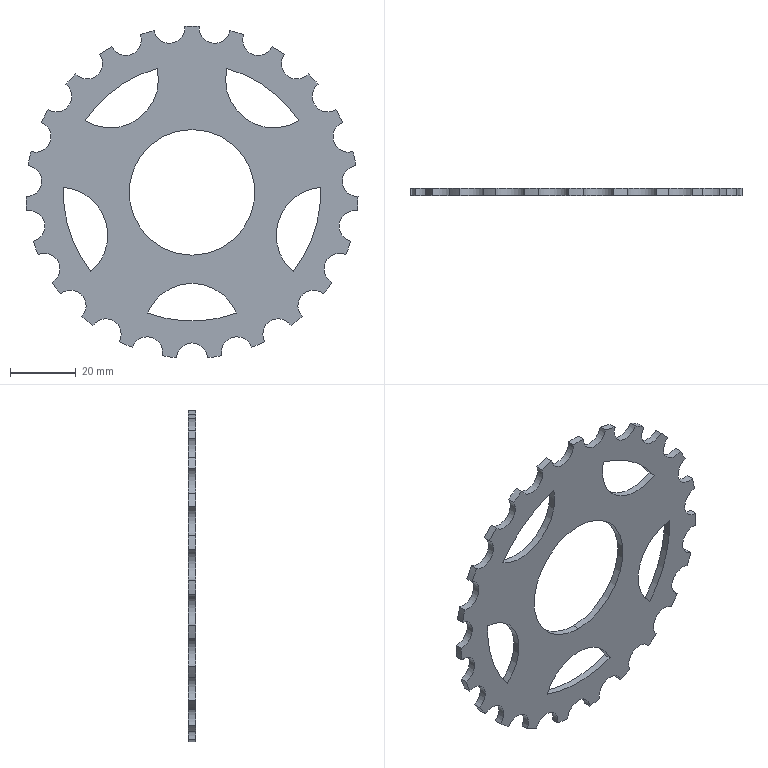Part | STEP file | Gear 2 | 1 solid | 72 faces | box 100.969 x 2.2 x 100.781 mm | volume 10960 mm3 | cylinder 70 | plane 2 | commonest cylinder face diameters 9.4 x34 101 x23 29.335 x6 78.243 x5 38.2 x2